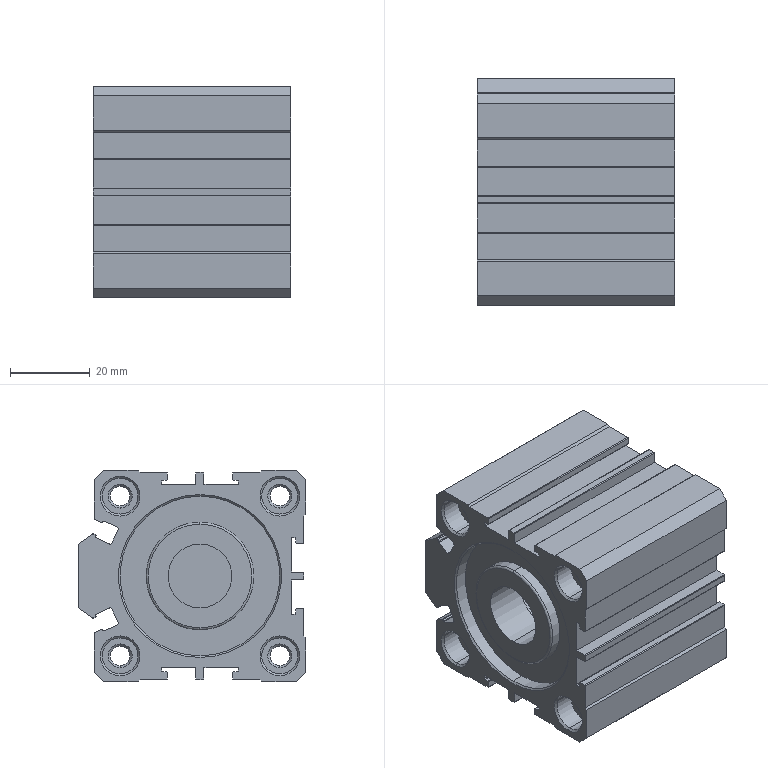Part | STEP file | 001-009-_ACQS-40x1010_b | 1 solid | 227 faces | box 49.5 x 57 x 53 mm | volume 74986 mm3 | cylinder 92 | plane 89 | cone 44 | torus 2 | commonest cylinder face diameters 0.4 x35 9 x16 0.8 x15 4.917 x8 40 x6 8.566 x4